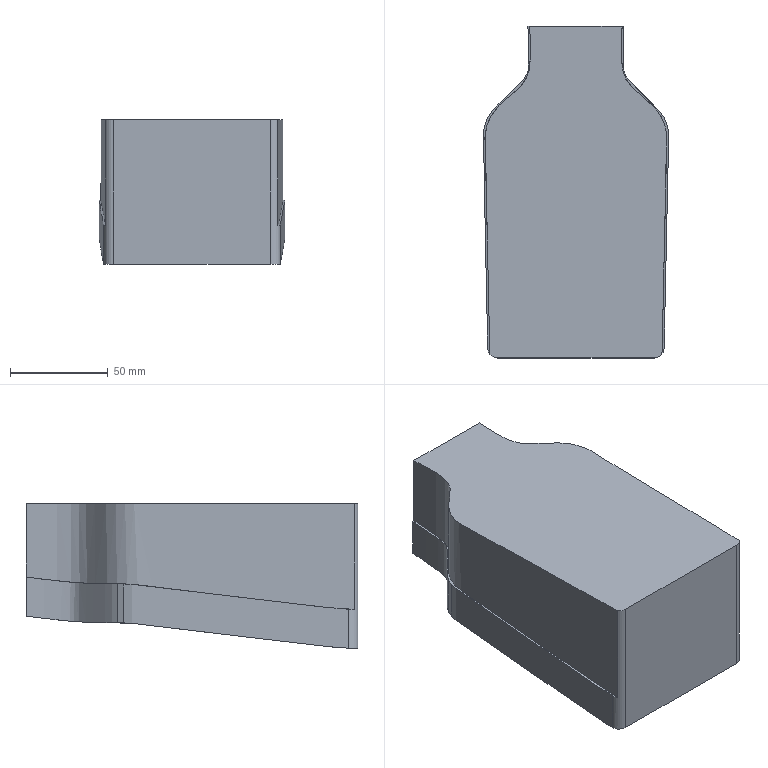Part | NX | features solid 2 | 1 solid | 16 faces | box 95.022 x 170 x 74.267 mm | volume 921105 mm3 | spline 11 | plane 3 | cylinder 2 | commonest cylinder face diameters 10 x2